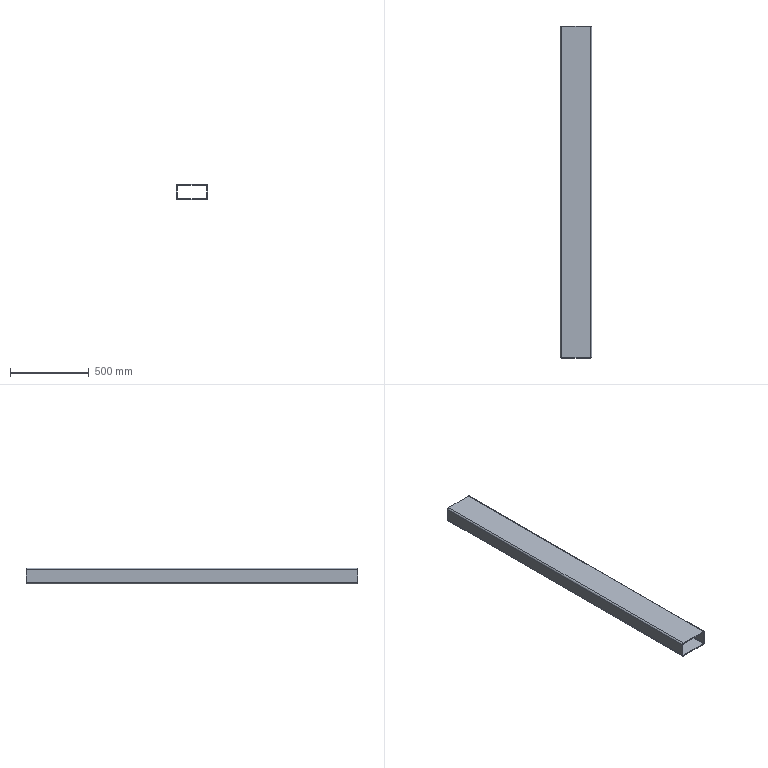Part | SolidWorks | features ExtruThin 1 | 1 solid | 18 faces | box 200 x 2114 x 100 mm | volume 7153551 mm3 | plane 10 | cylinder 8 | commonest cylinder face diameters 8 x4 20 x4
STEP:
#1=CARTESIAN_POINT('',(100.,1057.,-40.));
#2=VERTEX_POINT('',#1);
#3=CARTESIAN_POINT('',(90.,1057.,-50.));
#4=VERTEX_POINT('',#3);
#5=CARTESIAN_POINT('',(90.,1057.,-40.));
#6=DIRECTION('',(0.,1.,0.));
#7=DIRECTION('',(0.,0.,-1.));
#8=AXIS2_PLACEMENT_3D('',#5,#6,#7);
#9=CIRCLE('',#8,10.);
#10=EDGE_CURVE('',#2,#4,#9,.T.);
#11=ORIENTED_EDGE('',*,*,#10,.T.);
#12=CARTESIAN_POINT('',(-90.,1057.,-50.));
#13=VERTEX_POINT('',#12);
#14=CARTESIAN_POINT('',(-90.,1057.,-50.));
#15=DIRECTION('',(-1.,0.,0.));
#16=VECTOR('',#15,1000.);
#17=LINE('',#14,#16);
#18=EDGE_CURVE('',#4,#13,#17,.T.);
#19=ORIENTED_EDGE('',*,*,#18,.T.);
#20=CARTESIAN_POINT('',(-100.,1057.,-40.));
#21=VERTEX_POINT('',#20);
#22=CARTESIAN_POINT('',(-90.,1057.,-40.));
#23=DIRECTION('',(0.,1.,0.));
#24=DIRECTION('',(0.,0.,1.));
#25=AXIS2_PLACEMENT_3D('',#22,#23,#24);
#26=CIRCLE('',#25,10.);
#27=EDGE_CURVE('',#13,#21,#26,.T.);
#28=ORIENTED_EDGE('',*,*,#27,.T.);
#29=CARTESIAN_POINT('',(-100.,1057.,40.));
#30=VERTEX_POINT('',#29);
#31=CARTESIAN_POINT('',(-100.,1057.,-40.));
#32=DIRECTION('',(0.,0.,1.));
#33=VECTOR('',#32,1000.);
#34=LINE('',#31,#33);
#35=EDGE_CURVE('',#21,#30,#34,.T.);
#36=ORIENTED_EDGE('',*,*,#35,.T.);
#37=CARTESIAN_POINT('',(-90.,1057.,50.));
#38=VERTEX_POINT('',#37);
#39=CARTESIAN_POINT('',(-90.,1057.,40.));
#40=DIRECTION('',(0.,1.,0.));
#41=DIRECTION('',(0.,0.,1.));
#42=AXIS2_PLACEMENT_3D('',#39,#40,#41);
#43=CIRCLE('',#42,10.);
#44=EDGE_CURVE('',#30,#38,#43,.T.);
#45=ORIENTED_EDGE('',*,*,#44,.T.);
#46=CARTESIAN_POINT('',(90.,1057.,50.));
#47=VERTEX_POINT('',#46);
#48=CARTESIAN_POINT('',(-90.,1057.,50.));
#49=DIRECTION('',(1.,0.,0.));
#50=VECTOR('',#49,1000.);
#51=LINE('',#48,#50);
#52=EDGE_CURVE('',#38,#47,#51,.T.);
#53=ORIENTED_EDGE('',*,*,#52,.T.);
#54=CARTESIAN_POINT('',(100.,1057.,40.));
#55=VERTEX_POINT('',#54);
#56=CARTESIAN_POINT('',(90.,1057.,40.));
#57=DIRECTION('',(0.,1.,0.));
#58=DIRECTION('',(0.,0.,1.));
#59=AXIS2_PLACEMENT_3D('',#56,#57,#58);
#60=CIRCLE('',#59,10.);
#61=EDGE_CURVE('',#47,#55,#60,.T.);
#62=ORIENTED_EDGE('',*,*,#61,.T.);
#63=CARTESIAN_POINT('',(100.,1057.,-40.));
#64=DIRECTION('',(0.,0.,-1.));
#65=VECTOR('',#64,1000.);
#66=LINE('',#63,#65);
#67=EDGE_CURVE('',#55,#2,#66,.T.);
#68=ORIENTED_EDGE('',*,*,#67,.T.);
#69=EDGE_LOOP('',(#11,#19,#28,#36,#45,#53,#62,#68));
#70=FACE_OUTER_BOUND('',#69,.T.);
#71=CARTESIAN_POINT('',(90.,1057.,-44.));
#72=VERTEX_POINT('',#71);
#73=CARTESIAN_POINT('',(-90.,1057.,-44.));
#74=VERTEX_POINT('',#73);
#75=CARTESIAN_POINT('',(90.,1057.,-44.));
#76=DIRECTION('',(-1.,0.,0.));
#77=VECTOR('',#76,1000.);
#78=LINE('',#75,#77);
#79=EDGE_CURVE('',#72,#74,#78,.T.);
#80=ORIENTED_EDGE('',*,*,#79,.F.);
#81=CARTESIAN_POINT('',(94.,1057.,-40.));
#82=VERTEX_POINT('',#81);
#83=CARTESIAN_POINT('',(90.,1057.,-40.));
#84=DIRECTION('',(0.,1.,0.));
#85=DIRECTION('',(-1.,0.,0.));
#86=AXIS2_PLACEMENT_3D('',#83,#84,#85);
#87=CIRCLE('',#86,4.);
#88=EDGE_CURVE('',#82,#72,#87,.T.);
#89=ORIENTED_EDGE('',*,*,#88,.F.);
#90=CARTESIAN_POINT('',(94.,1057.,40.));
#91=VERTEX_POINT('',#90);
#92=CARTESIAN_POINT('',(94.,1057.,-40.));
#93=DIRECTION('',(0.,0.,-1.));
#94=VECTOR('',#93,1000.);
#95=LINE('',#92,#94);
#96=EDGE_CURVE('',#91,#82,#95,.T.);
#97=ORIENTED_EDGE('',*,*,#96,.F.);
#98=CARTESIAN_POINT('',(90.,1057.,44.));
#99=VERTEX_POINT('',#98);
#100=CARTESIAN_POINT('',(90.,1057.,40.));
#101=DIRECTION('',(0.,1.,0.));
#102=DIRECTION('',(-1.,0.,0.));
#103=AXIS2_PLACEMENT_3D('',#100,#101,#102);
#104=CIRCLE('',#103,4.);
#105=EDGE_CURVE('',#99,#91,#104,.T.);
#106=ORIENTED_EDGE('',*,*,#105,.F.);
#107=CARTESIAN_POINT('',(-90.,1057.,44.));
#108=VERTEX_POINT('',#107);
#109=CARTESIAN_POINT('',(90.,1057.,44.));
#110=DIRECTION('',(1.,0.,0.));
#111=VECTOR('',#110,1000.);
#112=LINE('',#109,#111);
#113=EDGE_CURVE('',#108,#99,#112,.T.);
#114=ORIENTED_EDGE('',*,*,#113,.F.);
#115=CARTESIAN_POINT('',(-94.,1057.,40.));
#116=VERTEX_POINT('',#115);
#117=CARTESIAN_POINT('',(-90.,1057.,40.));
#118=DIRECTION('',(0.,1.,0.));
#119=DIRECTION('',(-1.,0.,0.));
#120=AXIS2_PLACEMENT_3D('',#117,#118,#119);
#121=CIRCLE('',#120,4.);
#122=EDGE_CURVE('',#116,#108,#121,.T.);
#123=ORIENTED_EDGE('',*,*,#122,.F.);
#124=CARTESIAN_POINT('',(-94.,1057.,-40.));
#125=VERTEX_POINT('',#124);
#126=CARTESIAN_POINT('',(-94.,1057.,-40.));
#127=DIRECTION('',(0.,0.,1.));
#128=VECTOR('',#127,1000.);
#129=LINE('',#126,#128);
#130=EDGE_CURVE('',#125,#116,#129,.T.);
#131=ORIENTED_EDGE('',*,*,#130,.F.);
#132=CARTESIAN_POINT('',(-90.,1057.,-40.));
#133=DIRECTION('',(0.,1.,0.));
#134=DIRECTION('',(-1.,0.,0.));
#135=AXIS2_PLACEMENT_3D('',#132,#133,#134);
#136=CIRCLE('',#135,4.);
#137=EDGE_CURVE('',#74,#125,#136,.T.);
#138=ORIENTED_EDGE('',*,*,#137,.F.);
#139=EDGE_LOOP('',(#80,#89,#97,#106,#114,#123,#131,#138));
#140=FACE_BOUND('',#139,.T.);
#141=CARTESIAN_POINT('',(90.,1057.,-40.));
#142=DIRECTION('',(0.,1.,0.));
#143=DIRECTION('',(0.,0.,1.));
#144=AXIS2_PLACEMENT_3D('',#141,#142,#143);
#145=PLANE('',#144);
#146=ADVANCED_FACE('',(#70,#140),#145,.T.);
#147=CARTESIAN_POINT('',(100.,-1057.,-40.));
#148=VERTEX_POINT('',#147);
#149=CARTESIAN_POINT('',(90.,-1057.,-50.));
#150=VERTEX_POINT('',#149);
#151=CARTESIAN_POINT('',(90.,-1057.,-40.));
#152=DIRECTION('',(0.,1.,0.));
#153=DIRECTION('',(0.,0.,-1.));
#154=AXIS2_PLACEMENT_3D('',#151,#152,#153);
#155=CIRCLE('',#154,10.);
#156=EDGE_CURVE('',#148,#150,#155,.T.);
#157=ORIENTED_EDGE('',*,*,#156,.F.);
#158=CARTESIAN_POINT('',(100.,-1057.,40.));
#159=VERTEX_POINT('',#158);
#160=CARTESIAN_POINT('',(100.,-1057.,-40.));
#161=DIRECTION('',(0.,0.,-1.));
#162=VECTOR('',#161,1000.);
#163=LINE('',#160,#162);
#164=EDGE_CURVE('',#159,#148,#163,.T.);
#165=ORIENTED_EDGE('',*,*,#164,.F.);
#166=CARTESIAN_POINT('',(90.,-1057.,50.));
#167=VERTEX_POINT('',#166);
#168=CARTESIAN_POINT('',(90.,-1057.,40.));
#169=DIRECTION('',(0.,1.,0.));
#170=DIRECTION('',(0.,0.,1.));
#171=AXIS2_PLACEMENT_3D('',#168,#169,#170);
#172=CIRCLE('',#171,10.);
#173=EDGE_CURVE('',#167,#159,#172,.T.);
#174=ORIENTED_EDGE('',*,*,#173,.F.);
#175=CARTESIAN_POINT('',(-90.,-1057.,50.));
#176=VERTEX_POINT('',#175);
#177=CARTESIAN_POINT('',(-90.,-1057.,50.));
#178=DIRECTION('',(1.,0.,0.));
#179=VECTOR('',#178,1000.);
#180=LINE('',#177,#179);
#181=EDGE_CURVE('',#176,#167,#180,.T.);
#182=ORIENTED_EDGE('',*,*,#181,.F.);
#183=CARTESIAN_POINT('',(-100.,-1057.,40.));
#184=VERTEX_POINT('',#183);
#185=CARTESIAN_POINT('',(-90.,-1057.,40.));
#186=DIRECTION('',(0.,1.,0.));
#187=DIRECTION('',(0.,0.,1.));
#188=AXIS2_PLACEMENT_3D('',#185,#186,#187);
#189=CIRCLE('',#188,10.);
#190=EDGE_CURVE('',#184,#176,#189,.T.);
#191=ORIENTED_EDGE('',*,*,#190,.F.);
#192=CARTESIAN_POINT('',(-100.,-1057.,-40.));
#193=VERTEX_POINT('',#192);
#194=CARTESIAN_POINT('',(-100.,-1057.,-40.));
#195=DIRECTION('',(0.,0.,1.));
#196=VECTOR('',#195,1000.);
#197=LINE('',#194,#196);
#198=EDGE_CURVE('',#193,#184,#197,.T.);
#199=ORIENTED_EDGE('',*,*,#198,.F.);
#200=CARTESIAN_POINT('',(-90.,-1057.,-50.));
#201=VERTEX_POINT('',#200);
#202=CARTESIAN_POINT('',(-90.,-1057.,-40.));
#203=DIRECTION('',(0.,1.,0.));
#204=DIRECTION('',(0.,0.,1.));
#205=AXIS2_PLACEMENT_3D('',#202,#203,#204);
#206=CIRCLE('',#205,10.);
#207=EDGE_CURVE('',#201,#193,#206,.T.);
#208=ORIENTED_EDGE('',*,*,#207,.F.);
#209=CARTESIAN_POINT('',(-90.,-1057.,-50.));
#210=DIRECTION('',(-1.,0.,0.));
#211=VECTOR('',#210,1000.);
#212=LINE('',#209,#211);
#213=EDGE_CURVE('',#150,#201,#212,.T.);
#214=ORIENTED_EDGE('',*,*,#213,.F.);
#215=EDGE_LOOP('',(#157,#165,#174,#182,#191,#199,#208,#214));
#216=FACE_OUTER_BOUND('',#215,.T.);
#217=CARTESIAN_POINT('',(94.,-1057.,-40.));
#218=VERTEX_POINT('',#217);
#219=CARTESIAN_POINT('',(90.,-1057.,-44.));
#220=VERTEX_POINT('',#219);
#221=CARTESIAN_POINT('',(90.,-1057.,-40.));
#222=DIRECTION('',(0.,1.,0.));
#223=DIRECTION('',(-1.,0.,0.));
#224=AXIS2_PLACEMENT_3D('',#221,#222,#223);
#225=CIRCLE('',#224,4.);
#226=EDGE_CURVE('',#218,#220,#225,.T.);
#227=ORIENTED_EDGE('',*,*,#226,.T.);
#228=CARTESIAN_POINT('',(-90.,-1057.,-44.));
#229=VERTEX_POINT('',#228);
#230=CARTESIAN_POINT('',(90.,-1057.,-44.));
#231=DIRECTION('',(-1.,0.,0.));
#232=VECTOR('',#231,1000.);
#233=LINE('',#230,#232);
#234=EDGE_CURVE('',#220,#229,#233,.T.);
#235=ORIENTED_EDGE('',*,*,#234,.T.);
#236=CARTESIAN_POINT('',(-94.,-1057.,-40.));
#237=VERTEX_POINT('',#236);
#238=CARTESIAN_POINT('',(-90.,-1057.,-40.));
#239=DIRECTION('',(0.,1.,0.));
#240=DIRECTION('',(-1.,0.,0.));
#241=AXIS2_PLACEMENT_3D('',#238,#239,#240);
#242=CIRCLE('',#241,4.);
#243=EDGE_CURVE('',#229,#237,#242,.T.);
#244=ORIENTED_EDGE('',*,*,#243,.T.);
#245=CARTESIAN_POINT('',(-94.,-1057.,40.));
#246=VERTEX_POINT('',#245);
#247=CARTESIAN_POINT('',(-94.,-1057.,-40.));
#248=DIRECTION('',(0.,0.,1.));
#249=VECTOR('',#248,1000.);
#250=LINE('',#247,#249);
#251=EDGE_CURVE('',#237,#246,#250,.T.);
#252=ORIENTED_EDGE('',*,*,#251,.T.);
#253=CARTESIAN_POINT('',(-90.,-1057.,44.));
#254=VERTEX_POINT('',#253);
#255=CARTESIAN_POINT('',(-90.,-1057.,40.));
#256=DIRECTION('',(0.,1.,0.));
#257=DIRECTION('',(-1.,0.,0.));
#258=AXIS2_PLACEMENT_3D('',#255,#256,#257);
#259=CIRCLE('',#258,4.);
#260=EDGE_CURVE('',#246,#254,#259,.T.);
#261=ORIENTED_EDGE('',*,*,#260,.T.);
#262=CARTESIAN_POINT('',(90.,-1057.,44.));
#263=VERTEX_POINT('',#262);
#264=CARTESIAN_POINT('',(90.,-1057.,44.));
#265=DIRECTION('',(1.,0.,0.));
#266=VECTOR('',#265,1000.);
#267=LINE('',#264,#266);
#268=EDGE_CURVE('',#254,#263,#267,.T.);
#269=ORIENTED_EDGE('',*,*,#268,.T.);
#270=CARTESIAN_POINT('',(94.,-1057.,40.));
#271=VERTEX_POINT('',#270);
#272=CARTESIAN_POINT('',(90.,-1057.,40.));
#273=DIRECTION('',(0.,1.,0.));
#274=DIRECTION('',(-1.,0.,0.));
#275=AXIS2_PLACEMENT_3D('',#272,#273,#274);
#276=CIRCLE('',#275,4.);
#277=EDGE_CURVE('',#263,#271,#276,.T.);
#278=ORIENTED_EDGE('',*,*,#277,.T.);
#279=CARTESIAN_POINT('',(94.,-1057.,-40.));
#280=DIRECTION('',(0.,0.,-1.));
#281=VECTOR('',#280,1000.);
#282=LINE('',#279,#281);
#283=EDGE_CURVE('',#271,#218,#282,.T.);
#284=ORIENTED_EDGE('',*,*,#283,.T.);
#285=EDGE_LOOP('',(#227,#235,#244,#252,#261,#269,#278,#284));
#286=FACE_BOUND('',#285,.T.);
#287=CARTESIAN_POINT('',(90.,-1057.,-40.));
#288=DIRECTION('',(0.,1.,0.));
#289=DIRECTION('',(0.,0.,1.));
#290=AXIS2_PLACEMENT_3D('',#287,#288,#289);
#291=PLANE('',#290);
#292=ADVANCED_FACE('',(#216,#286),#291,.F.);
#293=ORIENTED_EDGE('',*,*,#156,.T.);
#294=CARTESIAN_POINT('',(90.,1057.,-50.));
#295=DIRECTION('',(0.,-1.,0.));
#296=VECTOR('',#295,1000.);
#297=LINE('',#294,#296);
#298=EDGE_CURVE('',#4,#150,#297,.T.);
#299=ORIENTED_EDGE('',*,*,#298,.F.);
#300=ORIENTED_EDGE('',*,*,#10,.F.);
#301=CARTESIAN_POINT('',(100.,1057.,-40.));
#302=DIRECTION('',(0.,-1.,0.));
#303=VECTOR('',#302,1000.);
#304=LINE('',#301,#303);
#305=EDGE_CURVE('',#2,#148,#304,.T.);
#306=ORIENTED_EDGE('',*,*,#305,.T.);
#307=EDGE_LOOP('',(#293,#299,#300,#306));
#308=FACE_OUTER_BOUND('',#307,.T.);
#309=CARTESIAN_POINT('',(90.,1057.,-40.));
#310=DIRECTION('',(0.,-1.,0.));
#311=DIRECTION('',(0.,0.,-1.));
#312=AXIS2_PLACEMENT_3D('',#309,#310,#311);
#313=CYLINDRICAL_SURFACE('',#312,10.);
#314=ADVANCED_FACE('',(#308),#313,.T.);
#315=ORIENTED_EDGE('',*,*,#213,.T.);
#316=CARTESIAN_POINT('',(-90.,1057.,-50.));
#317=DIRECTION('',(0.,-1.,0.));
#318=VECTOR('',#317,1000.);
#319=LINE('',#316,#318);
#320=EDGE_CURVE('',#13,#201,#319,.T.);
#321=ORIENTED_EDGE('',*,*,#320,.F.);
#322=ORIENTED_EDGE('',*,*,#18,.F.);
#323=ORIENTED_EDGE('',*,*,#298,.T.);
#324=EDGE_LOOP('',(#315,#321,#322,#323));
#325=FACE_OUTER_BOUND('',#324,.T.);
#326=CARTESIAN_POINT('',(-90.,1057.,-50.));
#327=DIRECTION('',(0.,0.,1.));
#328=DIRECTION('',(1.,0.,0.));
#329=AXIS2_PLACEMENT_3D('',#326,#327,#328);
#330=PLANE('',#329);
#331=ADVANCED_FACE('',(#325),#330,.F.);
#332=ORIENTED_EDGE('',*,*,#207,.T.);
#333=CARTESIAN_POINT('',(-100.,1057.,-40.));
#334=DIRECTION('',(0.,-1.,0.));
#335=VECTOR('',#334,1000.);
#336=LINE('',#333,#335);
#337=EDGE_CURVE('',#21,#193,#336,.T.);
#338=ORIENTED_EDGE('',*,*,#337,.F.);
#339=ORIENTED_EDGE('',*,*,#27,.F.);
#340=ORIENTED_EDGE('',*,*,#320,.T.);
#341=EDGE_LOOP('',(#332,#338,#339,#340));
#342=FACE_OUTER_BOUND('',#341,.T.);
#343=CARTESIAN_POINT('',(-90.,1057.,-40.));
#344=DIRECTION('',(0.,-1.,0.));
#345=DIRECTION('',(0.,0.,-1.));
#346=AXIS2_PLACEMENT_3D('',#343,#344,#345);
#347=CYLINDRICAL_SURFACE('',#346,10.);
#348=ADVANCED_FACE('',(#342),#347,.T.);
#349=ORIENTED_EDGE('',*,*,#198,.T.);
#350=CARTESIAN_POINT('',(-100.,1057.,40.));
#351=DIRECTION('',(0.,-1.,0.));
#352=VECTOR('',#351,1000.);
#353=LINE('',#350,#352);
#354=EDGE_CURVE('',#30,#184,#353,.T.);
#355=ORIENTED_EDGE('',*,*,#354,.F.);
#356=ORIENTED_EDGE('',*,*,#35,.F.);
#357=ORIENTED_EDGE('',*,*,#337,.T.);
#358=EDGE_LOOP('',(#349,#355,#356,#357));
#359=FACE_OUTER_BOUND('',#358,.T.);
#360=CARTESIAN_POINT('',(-100.,1057.,-40.));
#361=DIRECTION('',(1.,0.,0.));
#362=DIRECTION('',(0.,0.,-1.));
#363=AXIS2_PLACEMENT_3D('',#360,#361,#362);
#364=PLANE('',#363);
#365=ADVANCED_FACE('',(#359),#364,.F.);
#366=ORIENTED_EDGE('',*,*,#190,.T.);
#367=CARTESIAN_POINT('',(-90.,1057.,50.));
#368=DIRECTION('',(0.,-1.,0.));
#369=VECTOR('',#368,1000.);
#370=LINE('',#367,#369);
#371=EDGE_CURVE('',#38,#176,#370,.T.);
#372=ORIENTED_EDGE('',*,*,#371,.F.);
#373=ORIENTED_EDGE('',*,*,#44,.F.);
#374=ORIENTED_EDGE('',*,*,#354,.T.);
#375=EDGE_LOOP('',(#366,#372,#373,#374));
#376=FACE_OUTER_BOUND('',#375,.T.);
#377=CARTESIAN_POINT('',(-90.,1057.,40.));
#378=DIRECTION('',(0.,-1.,0.));
#379=DIRECTION('',(0.,0.,-1.));
#380=AXIS2_PLACEMENT_3D('',#377,#378,#379);
#381=CYLINDRICAL_SURFACE('',#380,10.);
#382=ADVANCED_FACE('',(#376),#381,.T.);
#383=ORIENTED_EDGE('',*,*,#181,.T.);
#384=CARTESIAN_POINT('',(90.,1057.,50.));
#385=DIRECTION('',(0.,-1.,0.));
#386=VECTOR('',#385,1000.);
#387=LINE('',#384,#386);
#388=EDGE_CURVE('',#47,#167,#387,.T.);
#389=ORIENTED_EDGE('',*,*,#388,.F.);
#390=ORIENTED_EDGE('',*,*,#52,.F.);
#391=ORIENTED_EDGE('',*,*,#371,.T.);
#392=EDGE_LOOP('',(#383,#389,#390,#391));
#393=FACE_OUTER_BOUND('',#392,.T.);
#394=CARTESIAN_POINT('',(-90.,1057.,50.));
#395=DIRECTION('',(0.,0.,-1.));
#396=DIRECTION('',(-1.,0.,0.));
#397=AXIS2_PLACEMENT_3D('',#394,#395,#396);
#398=PLANE('',#397);
#399=ADVANCED_FACE('',(#393),#398,.F.);
#400=ORIENTED_EDGE('',*,*,#173,.T.);
#401=CARTESIAN_POINT('',(100.,1057.,40.));
#402=DIRECTION('',(0.,-1.,0.));
#403=VECTOR('',#402,1000.);
#404=LINE('',#401,#403);
#405=EDGE_CURVE('',#55,#159,#404,.T.);
#406=ORIENTED_EDGE('',*,*,#405,.F.);
#407=ORIENTED_EDGE('',*,*,#61,.F.);
#408=ORIENTED_EDGE('',*,*,#388,.T.);
#409=EDGE_LOOP('',(#400,#406,#407,#408));
#410=FACE_OUTER_BOUND('',#409,.T.);
#411=CARTESIAN_POINT('',(90.,1057.,40.));
#412=DIRECTION('',(0.,-1.,0.));
#413=DIRECTION('',(0.,0.,-1.));
#414=AXIS2_PLACEMENT_3D('',#411,#412,#413);
#415=CYLINDRICAL_SURFACE('',#414,10.);
#416=ADVANCED_FACE('',(#410),#415,.T.);
#417=ORIENTED_EDGE('',*,*,#164,.T.);
#418=ORIENTED_EDGE('',*,*,#305,.F.);
#419=ORIENTED_EDGE('',*,*,#67,.F.);
#420=ORIENTED_EDGE('',*,*,#405,.T.);
#421=EDGE_LOOP('',(#417,#418,#419,#420));
#422=FACE_OUTER_BOUND('',#421,.T.);
#423=CARTESIAN_POINT('',(100.,1057.,-40.));
#424=DIRECTION('',(-1.,0.,0.));
#425=DIRECTION('',(0.,0.,1.));
#426=AXIS2_PLACEMENT_3D('',#423,#424,#425);
#427=PLANE('',#426);
#428=ADVANCED_FACE('',(#422),#427,.F.);
#429=ORIENTED_EDGE('',*,*,#226,.F.);
#430=CARTESIAN_POINT('',(94.,1057.,-40.));
#431=DIRECTION('',(0.,-1.,0.));
#432=VECTOR('',#431,1000.);
#433=LINE('',#430,#432);
#434=EDGE_CURVE('',#82,#218,#433,.T.);
#435=ORIENTED_EDGE('',*,*,#434,.F.);
#436=ORIENTED_EDGE('',*,*,#88,.T.);
#437=CARTESIAN_POINT('',(90.,1057.,-44.));
#438=DIRECTION('',(0.,-1.,0.));
#439=VECTOR('',#438,1000.);
#440=LINE('',#437,#439);
#441=EDGE_CURVE('',#72,#220,#440,.T.);
#442=ORIENTED_EDGE('',*,*,#441,.T.);
#443=EDGE_LOOP('',(#429,#435,#436,#442));
#444=FACE_OUTER_BOUND('',#443,.T.);
#445=CARTESIAN_POINT('',(90.,1057.,-40.));
#446=DIRECTION('',(0.,-1.,0.));
#447=DIRECTION('',(0.,0.,-1.));
#448=AXIS2_PLACEMENT_3D('',#445,#446,#447);
#449=CYLINDRICAL_SURFACE('',#448,4.);
#450=ADVANCED_FACE('',(#444),#449,.F.);
#451=ORIENTED_EDGE('',*,*,#234,.F.);
#452=ORIENTED_EDGE('',*,*,#441,.F.);
#453=ORIENTED_EDGE('',*,*,#79,.T.);
#454=CARTESIAN_POINT('',(-90.,1057.,-44.));
#455=DIRECTION('',(0.,-1.,0.));
#456=VECTOR('',#455,1000.);
#457=LINE('',#454,#456);
#458=EDGE_CURVE('',#74,#229,#457,.T.);
#459=ORIENTED_EDGE('',*,*,#458,.T.);
#460=EDGE_LOOP('',(#451,#452,#453,#459));
#461=FACE_OUTER_BOUND('',#460,.T.);
#462=CARTESIAN_POINT('',(90.,1057.,-44.));
#463=DIRECTION('',(0.,0.,1.));
#464=DIRECTION('',(1.,0.,0.));
#465=AXIS2_PLACEMENT_3D('',#462,#463,#464);
#466=PLANE('',#465);
#467=ADVANCED_FACE('',(#461),#466,.T.);
#468=ORIENTED_EDGE('',*,*,#243,.F.);
#469=ORIENTED_EDGE('',*,*,#458,.F.);
#470=ORIENTED_EDGE('',*,*,#137,.T.);
#471=CARTESIAN_POINT('',(-94.,1057.,-40.));
#472=DIRECTION('',(0.,-1.,0.));
#473=VECTOR('',#472,1000.);
#474=LINE('',#471,#473);
#475=EDGE_CURVE('',#125,#237,#474,.T.);
#476=ORIENTED_EDGE('',*,*,#475,.T.);
#477=EDGE_LOOP('',(#468,#469,#470,#476));
#478=FACE_OUTER_BOUND('',#477,.T.);
#479=CARTESIAN_POINT('',(-90.,1057.,-40.));
#480=DIRECTION('',(0.,-1.,0.));
#481=DIRECTION('',(0.,0.,-1.));
#482=AXIS2_PLACEMENT_3D('',#479,#480,#481);
#483=CYLINDRICAL_SURFACE('',#482,4.);
#484=ADVANCED_FACE('',(#478),#483,.F.);
#485=ORIENTED_EDGE('',*,*,#251,.F.);
#486=ORIENTED_EDGE('',*,*,#475,.F.);
#487=ORIENTED_EDGE('',*,*,#130,.T.);
#488=CARTESIAN_POINT('',(-94.,1057.,40.));
#489=DIRECTION('',(0.,-1.,0.));
#490=VECTOR('',#489,1000.);
#491=LINE('',#488,#490);
#492=EDGE_CURVE('',#116,#246,#491,.T.);
#493=ORIENTED_EDGE('',*,*,#492,.T.);
#494=EDGE_LOOP('',(#485,#486,#487,#493));
#495=FACE_OUTER_BOUND('',#494,.T.);
#496=CARTESIAN_POINT('',(-94.,1057.,-40.));
#497=DIRECTION('',(1.,0.,0.));
#498=DIRECTION('',(0.,0.,-1.));
#499=AXIS2_PLACEMENT_3D('',#496,#497,#498);
#500=PLANE('',#499);
#501=ADVANCED_FACE('',(#495),#500,.T.);
#502=ORIENTED_EDGE('',*,*,#260,.F.);
#503=ORIENTED_EDGE('',*,*,#492,.F.);
#504=ORIENTED_EDGE('',*,*,#122,.T.);
#505=CARTESIAN_POINT('',(-90.,1057.,44.));
#506=DIRECTION('',(0.,-1.,0.));
#507=VECTOR('',#506,1000.);
#508=LINE('',#505,#507);
#509=EDGE_CURVE('',#108,#254,#508,.T.);
#510=ORIENTED_EDGE('',*,*,#509,.T.);
#511=EDGE_LOOP('',(#502,#503,#504,#510));
#512=FACE_OUTER_BOUND('',#511,.T.);
#513=CARTESIAN_POINT('',(-90.,1057.,40.));
#514=DIRECTION('',(0.,-1.,0.));
#515=DIRECTION('',(0.,0.,-1.));
#516=AXIS2_PLACEMENT_3D('',#513,#514,#515);
#517=CYLINDRICAL_SURFACE('',#516,4.);
#518=ADVANCED_FACE('',(#512),#517,.F.);
#519=ORIENTED_EDGE('',*,*,#268,.F.);
#520=ORIENTED_EDGE('',*,*,#509,.F.);
#521=ORIENTED_EDGE('',*,*,#113,.T.);
#522=CARTESIAN_POINT('',(90.,1057.,44.));
#523=DIRECTION('',(0.,-1.,0.));
#524=VECTOR('',#523,1000.);
#525=LINE('',#522,#524);
#526=EDGE_CURVE('',#99,#263,#525,.T.);
#527=ORIENTED_EDGE('',*,*,#526,.T.);
#528=EDGE_LOOP('',(#519,#520,#521,#527));
#529=FACE_OUTER_BOUND('',#528,.T.);
#530=CARTESIAN_POINT('',(90.,1057.,44.));
#531=DIRECTION('',(0.,0.,-1.));
#532=DIRECTION('',(-1.,0.,0.));
#533=AXIS2_PLACEMENT_3D('',#530,#531,#532);
#534=PLANE('',#533);
#535=ADVANCED_FACE('',(#529),#534,.T.);
#536=ORIENTED_EDGE('',*,*,#277,.F.);
#537=ORIENTED_EDGE('',*,*,#526,.F.);
#538=ORIENTED_EDGE('',*,*,#105,.T.);
#539=CARTESIAN_POINT('',(94.,1057.,40.));
#540=DIRECTION('',(0.,-1.,0.));
#541=VECTOR('',#540,1000.);
#542=LINE('',#539,#541);
#543=EDGE_CURVE('',#91,#271,#542,.T.);
#544=ORIENTED_EDGE('',*,*,#543,.T.);
#545=EDGE_LOOP('',(#536,#537,#538,#544));
#546=FACE_OUTER_BOUND('',#545,.T.);
#547=CARTESIAN_POINT('',(90.,1057.,40.));
#548=DIRECTION('',(0.,-1.,0.));
#549=DIRECTION('',(0.,0.,-1.));
#550=AXIS2_PLACEMENT_3D('',#547,#548,#549);
#551=CYLINDRICAL_SURFACE('',#550,4.);
#552=ADVANCED_FACE('',(#546),#551,.F.);
#553=ORIENTED_EDGE('',*,*,#283,.F.);
#554=ORIENTED_EDGE('',*,*,#543,.F.);
#555=ORIENTED_EDGE('',*,*,#96,.T.);
#556=ORIENTED_EDGE('',*,*,#434,.T.);
#557=EDGE_LOOP('',(#553,#554,#555,#556));
#558=FACE_OUTER_BOUND('',#557,.T.);
#559=CARTESIAN_POINT('',(94.,1057.,-40.));
#560=DIRECTION('',(-1.,0.,0.));
#561=DIRECTION('',(0.,0.,1.));
#562=AXIS2_PLACEMENT_3D('',#559,#560,#561);
#563=PLANE('',#562);
#564=ADVANCED_FACE('',(#558),#563,.T.);
#565=CLOSED_SHELL('',(#146,#292,#314,#331,#348,#365,#382,#399,#416,#428,#450,#467,#484,#501,#518,#535,#552,#564));
#566=MANIFOLD_SOLID_BREP('',#565);
#567=CARTESIAN_POINT('',(0.,0.,0.));
#568=DIRECTION('',(0.,0.,1.));
#569=DIRECTION('',(1.,0.,0.));
#570=AXIS2_PLACEMENT_3D('',#567,#568,#569);
#571=(LENGTH_UNIT()NAMED_UNIT(*)SI_UNIT(.MILLI.,.METRE.));
#572=UNCERTAINTY_MEASURE_WITH_UNIT(LENGTH_MEASURE(0.00001),#571,'','');
#573=(NAMED_UNIT(*)PLANE_ANGLE_UNIT()SI_UNIT($,.RADIAN.));
#574=(NAMED_UNIT(*)SI_UNIT($,.STERADIAN.)SOLID_ANGLE_UNIT());
#575=(GEOMETRIC_REPRESENTATION_CONTEXT(3)GLOBAL_UNCERTAINTY_ASSIGNED_CONTEXT((#572))GLOBAL_UNIT_ASSIGNED_CONTEXT((#571,#573,#574))REPRESENTATION_CONTEXT('',''));
#576=ADVANCED_BREP_SHAPE_REPRESENTATION('',(#566,#570),#575);